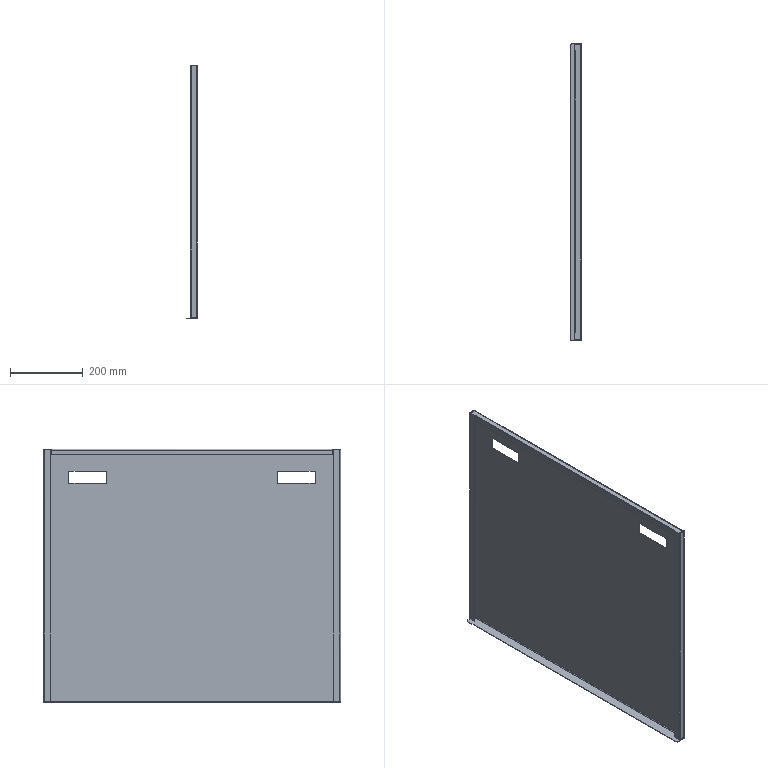Part | STEP file | MANIFOLD_SOLID_BREP_304524-2 | 1 solid | 62 faces | box 30 x 816 x 696 mm | volume 984068 mm3 | plane 46 | cylinder 16 | commonest cylinder face diameters 3 x7 6 x7 10 x2